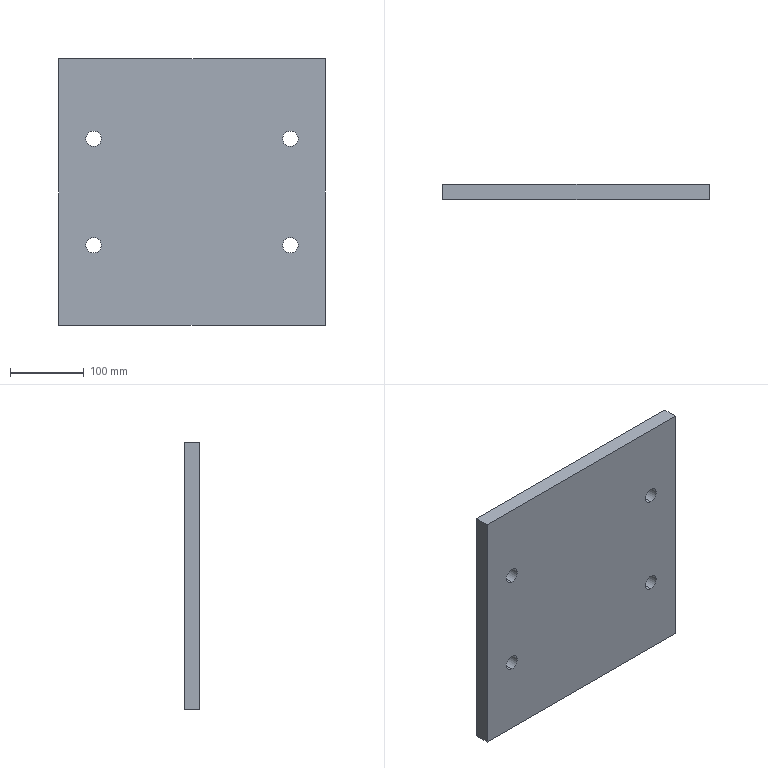Part | SolidWorks | features Extrusion 1, HoleWzd 1, LPattern 1 | 1 solid | 14 faces | box 360 x 20 x 360 mm | volume 2564291 mm3 | cylinder 8 | plane 6 | commonest cylinder face diameters 21 x8
STEP:
#1=CARTESIAN_POINT('',(133.,-10.,61.5));
#2=VERTEX_POINT('',#1);
#3=CARTESIAN_POINT('',(133.,-10.,82.5));
#4=VERTEX_POINT('',#3);
#5=CARTESIAN_POINT('',(133.,-10.,72.));
#6=DIRECTION('',(0.,1.,0.));
#7=DIRECTION('',(0.,0.,1.));
#8=AXIS2_PLACEMENT_3D('',#5,#6,#7);
#9=CIRCLE('',#8,10.5);
#10=EDGE_CURVE('',#2,#4,#9,.T.);
#11=ORIENTED_EDGE('',*,*,#10,.F.);
#12=CARTESIAN_POINT('',(133.,10.,61.5));
#13=VERTEX_POINT('',#12);
#14=CARTESIAN_POINT('',(133.,10.,61.5));
#15=DIRECTION('',(0.,1.,0.));
#16=VECTOR('',#15,1000.);
#17=LINE('',#14,#16);
#18=EDGE_CURVE('',#2,#13,#17,.T.);
#19=ORIENTED_EDGE('',*,*,#18,.T.);
#20=CARTESIAN_POINT('',(133.,10.,82.5));
#21=VERTEX_POINT('',#20);
#22=CARTESIAN_POINT('',(133.,10.,72.));
#23=DIRECTION('',(0.,1.,0.));
#24=DIRECTION('',(0.,0.,1.));
#25=AXIS2_PLACEMENT_3D('',#22,#23,#24);
#26=CIRCLE('',#25,10.5);
#27=EDGE_CURVE('',#13,#21,#26,.T.);
#28=ORIENTED_EDGE('',*,*,#27,.T.);
#29=CARTESIAN_POINT('',(133.,10.,82.5));
#30=DIRECTION('',(0.,1.,0.));
#31=VECTOR('',#30,1000.);
#32=LINE('',#29,#31);
#33=EDGE_CURVE('',#4,#21,#32,.T.);
#34=ORIENTED_EDGE('',*,*,#33,.F.);
#35=EDGE_LOOP('',(#11,#19,#28,#34));
#36=FACE_OUTER_BOUND('',#35,.T.);
#37=CARTESIAN_POINT('',(133.,10.,72.));
#38=DIRECTION('',(0.,1.,0.));
#39=DIRECTION('',(0.,0.,1.));
#40=AXIS2_PLACEMENT_3D('',#37,#38,#39);
#41=CYLINDRICAL_SURFACE('',#40,10.5);
#42=ADVANCED_FACE('',(#36),#41,.F.);
#43=CARTESIAN_POINT('',(133.,-10.,-82.5));
#44=VERTEX_POINT('',#43);
#45=CARTESIAN_POINT('',(133.,-10.,-61.5));
#46=VERTEX_POINT('',#45);
#47=CARTESIAN_POINT('',(133.,-10.,-72.));
#48=DIRECTION('',(0.,1.,0.));
#49=DIRECTION('',(0.,0.,1.));
#50=AXIS2_PLACEMENT_3D('',#47,#48,#49);
#51=CIRCLE('',#50,10.5);
#52=EDGE_CURVE('',#44,#46,#51,.T.);
#53=ORIENTED_EDGE('',*,*,#52,.F.);
#54=CARTESIAN_POINT('',(133.,10.,-82.5));
#55=VERTEX_POINT('',#54);
#56=CARTESIAN_POINT('',(133.,10.,-82.5));
#57=DIRECTION('',(0.,1.,0.));
#58=VECTOR('',#57,1000.);
#59=LINE('',#56,#58);
#60=EDGE_CURVE('',#44,#55,#59,.T.);
#61=ORIENTED_EDGE('',*,*,#60,.T.);
#62=CARTESIAN_POINT('',(133.,10.,-61.5));
#63=VERTEX_POINT('',#62);
#64=CARTESIAN_POINT('',(133.,10.,-72.));
#65=DIRECTION('',(0.,1.,0.));
#66=DIRECTION('',(0.,0.,1.));
#67=AXIS2_PLACEMENT_3D('',#64,#65,#66);
#68=CIRCLE('',#67,10.5);
#69=EDGE_CURVE('',#55,#63,#68,.T.);
#70=ORIENTED_EDGE('',*,*,#69,.T.);
#71=CARTESIAN_POINT('',(133.,10.,-61.5));
#72=DIRECTION('',(0.,1.,0.));
#73=VECTOR('',#72,1000.);
#74=LINE('',#71,#73);
#75=EDGE_CURVE('',#46,#63,#74,.T.);
#76=ORIENTED_EDGE('',*,*,#75,.F.);
#77=EDGE_LOOP('',(#53,#61,#70,#76));
#78=FACE_OUTER_BOUND('',#77,.T.);
#79=CARTESIAN_POINT('',(133.,10.,-72.));
#80=DIRECTION('',(0.,1.,0.));
#81=DIRECTION('',(0.,0.,1.));
#82=AXIS2_PLACEMENT_3D('',#79,#80,#81);
#83=CYLINDRICAL_SURFACE('',#82,10.5);
#84=ADVANCED_FACE('',(#78),#83,.F.);
#85=CARTESIAN_POINT('',(-133.,-10.,61.5));
#86=VERTEX_POINT('',#85);
#87=CARTESIAN_POINT('',(-133.,-10.,82.5));
#88=VERTEX_POINT('',#87);
#89=CARTESIAN_POINT('',(-133.,-10.,72.));
#90=DIRECTION('',(0.,1.,0.));
#91=DIRECTION('',(0.,0.,1.));
#92=AXIS2_PLACEMENT_3D('',#89,#90,#91);
#93=CIRCLE('',#92,10.5);
#94=EDGE_CURVE('',#86,#88,#93,.T.);
#95=ORIENTED_EDGE('',*,*,#94,.F.);
#96=CARTESIAN_POINT('',(-133.,10.,61.5));
#97=VERTEX_POINT('',#96);
#98=CARTESIAN_POINT('',(-133.,10.,61.5));
#99=DIRECTION('',(0.,1.,0.));
#100=VECTOR('',#99,1000.);
#101=LINE('',#98,#100);
#102=EDGE_CURVE('',#86,#97,#101,.T.);
#103=ORIENTED_EDGE('',*,*,#102,.T.);
#104=CARTESIAN_POINT('',(-133.,10.,82.5));
#105=VERTEX_POINT('',#104);
#106=CARTESIAN_POINT('',(-133.,10.,72.));
#107=DIRECTION('',(0.,1.,0.));
#108=DIRECTION('',(0.,0.,1.));
#109=AXIS2_PLACEMENT_3D('',#106,#107,#108);
#110=CIRCLE('',#109,10.5);
#111=EDGE_CURVE('',#97,#105,#110,.T.);
#112=ORIENTED_EDGE('',*,*,#111,.T.);
#113=CARTESIAN_POINT('',(-133.,10.,82.5));
#114=DIRECTION('',(0.,1.,0.));
#115=VECTOR('',#114,1000.);
#116=LINE('',#113,#115);
#117=EDGE_CURVE('',#88,#105,#116,.T.);
#118=ORIENTED_EDGE('',*,*,#117,.F.);
#119=EDGE_LOOP('',(#95,#103,#112,#118));
#120=FACE_OUTER_BOUND('',#119,.T.);
#121=CARTESIAN_POINT('',(-133.,10.,72.));
#122=DIRECTION('',(0.,1.,0.));
#123=DIRECTION('',(0.,0.,1.));
#124=AXIS2_PLACEMENT_3D('',#121,#122,#123);
#125=CYLINDRICAL_SURFACE('',#124,10.5);
#126=ADVANCED_FACE('',(#120),#125,.F.);
#127=CARTESIAN_POINT('',(-133.,-10.,-82.5));
#128=VERTEX_POINT('',#127);
#129=CARTESIAN_POINT('',(-133.,-10.,-61.5));
#130=VERTEX_POINT('',#129);
#131=CARTESIAN_POINT('',(-133.,-10.,-72.));
#132=DIRECTION('',(0.,1.,0.));
#133=DIRECTION('',(0.,0.,1.));
#134=AXIS2_PLACEMENT_3D('',#131,#132,#133);
#135=CIRCLE('',#134,10.5);
#136=EDGE_CURVE('',#128,#130,#135,.T.);
#137=ORIENTED_EDGE('',*,*,#136,.F.);
#138=CARTESIAN_POINT('',(-133.,10.,-82.5));
#139=VERTEX_POINT('',#138);
#140=CARTESIAN_POINT('',(-133.,10.,-82.5));
#141=DIRECTION('',(0.,1.,0.));
#142=VECTOR('',#141,1000.);
#143=LINE('',#140,#142);
#144=EDGE_CURVE('',#128,#139,#143,.T.);
#145=ORIENTED_EDGE('',*,*,#144,.T.);
#146=CARTESIAN_POINT('',(-133.,10.,-61.5));
#147=VERTEX_POINT('',#146);
#148=CARTESIAN_POINT('',(-133.,10.,-72.));
#149=DIRECTION('',(0.,1.,0.));
#150=DIRECTION('',(0.,0.,1.));
#151=AXIS2_PLACEMENT_3D('',#148,#149,#150);
#152=CIRCLE('',#151,10.5);
#153=EDGE_CURVE('',#139,#147,#152,.T.);
#154=ORIENTED_EDGE('',*,*,#153,.T.);
#155=CARTESIAN_POINT('',(-133.,10.,-61.5));
#156=DIRECTION('',(0.,1.,0.));
#157=VECTOR('',#156,1000.);
#158=LINE('',#155,#157);
#159=EDGE_CURVE('',#130,#147,#158,.T.);
#160=ORIENTED_EDGE('',*,*,#159,.F.);
#161=EDGE_LOOP('',(#137,#145,#154,#160));
#162=FACE_OUTER_BOUND('',#161,.T.);
#163=CARTESIAN_POINT('',(-133.,10.,-72.));
#164=DIRECTION('',(0.,1.,0.));
#165=DIRECTION('',(0.,0.,1.));
#166=AXIS2_PLACEMENT_3D('',#163,#164,#165);
#167=CYLINDRICAL_SURFACE('',#166,10.5);
#168=ADVANCED_FACE('',(#162),#167,.F.);
#169=CARTESIAN_POINT('',(180.,-10.,-180.));
#170=VERTEX_POINT('',#169);
#171=CARTESIAN_POINT('',(-180.,-10.,-180.));
#172=VERTEX_POINT('',#171);
#173=CARTESIAN_POINT('',(180.,-10.,-180.));
#174=DIRECTION('',(-1.,0.,0.));
#175=VECTOR('',#174,1000.);
#176=LINE('',#173,#175);
#177=EDGE_CURVE('',#170,#172,#176,.T.);
#178=ORIENTED_EDGE('',*,*,#177,.T.);
#179=CARTESIAN_POINT('',(-180.,10.,-180.));
#180=VERTEX_POINT('',#179);
#181=CARTESIAN_POINT('',(-180.,10.,-180.));
#182=DIRECTION('',(0.,-1.,0.));
#183=VECTOR('',#182,1000.);
#184=LINE('',#181,#183);
#185=EDGE_CURVE('',#180,#172,#184,.T.);
#186=ORIENTED_EDGE('',*,*,#185,.F.);
#187=CARTESIAN_POINT('',(180.,10.,-180.));
#188=VERTEX_POINT('',#187);
#189=CARTESIAN_POINT('',(180.,10.,-180.));
#190=DIRECTION('',(-1.,0.,0.));
#191=VECTOR('',#190,1000.);
#192=LINE('',#189,#191);
#193=EDGE_CURVE('',#188,#180,#192,.T.);
#194=ORIENTED_EDGE('',*,*,#193,.F.);
#195=CARTESIAN_POINT('',(180.,10.,-180.));
#196=DIRECTION('',(0.,-1.,0.));
#197=VECTOR('',#196,1000.);
#198=LINE('',#195,#197);
#199=EDGE_CURVE('',#188,#170,#198,.T.);
#200=ORIENTED_EDGE('',*,*,#199,.T.);
#201=EDGE_LOOP('',(#178,#186,#194,#200));
#202=FACE_OUTER_BOUND('',#201,.T.);
#203=CARTESIAN_POINT('',(180.,10.,-180.));
#204=DIRECTION('',(0.,0.,1.));
#205=DIRECTION('',(1.,0.,0.));
#206=AXIS2_PLACEMENT_3D('',#203,#204,#205);
#207=PLANE('',#206);
#208=ADVANCED_FACE('',(#202),#207,.F.);
#209=CARTESIAN_POINT('',(-180.,-10.,180.));
#210=VERTEX_POINT('',#209);
#211=CARTESIAN_POINT('',(-180.,-10.,-180.));
#212=DIRECTION('',(0.,0.,1.));
#213=VECTOR('',#212,1000.);
#214=LINE('',#211,#213);
#215=EDGE_CURVE('',#172,#210,#214,.T.);
#216=ORIENTED_EDGE('',*,*,#215,.T.);
#217=CARTESIAN_POINT('',(-180.,10.,180.));
#218=VERTEX_POINT('',#217);
#219=CARTESIAN_POINT('',(-180.,10.,180.));
#220=DIRECTION('',(0.,-1.,0.));
#221=VECTOR('',#220,1000.);
#222=LINE('',#219,#221);
#223=EDGE_CURVE('',#218,#210,#222,.T.);
#224=ORIENTED_EDGE('',*,*,#223,.F.);
#225=CARTESIAN_POINT('',(-180.,10.,-180.));
#226=DIRECTION('',(0.,0.,1.));
#227=VECTOR('',#226,1000.);
#228=LINE('',#225,#227);
#229=EDGE_CURVE('',#180,#218,#228,.T.);
#230=ORIENTED_EDGE('',*,*,#229,.F.);
#231=ORIENTED_EDGE('',*,*,#185,.T.);
#232=EDGE_LOOP('',(#216,#224,#230,#231));
#233=FACE_OUTER_BOUND('',#232,.T.);
#234=CARTESIAN_POINT('',(-180.,10.,-180.));
#235=DIRECTION('',(1.,0.,0.));
#236=DIRECTION('',(0.,0.,-1.));
#237=AXIS2_PLACEMENT_3D('',#234,#235,#236);
#238=PLANE('',#237);
#239=ADVANCED_FACE('',(#233),#238,.F.);
#240=CARTESIAN_POINT('',(180.,-10.,180.));
#241=VERTEX_POINT('',#240);
#242=CARTESIAN_POINT('',(-180.,-10.,180.));
#243=DIRECTION('',(1.,0.,0.));
#244=VECTOR('',#243,1000.);
#245=LINE('',#242,#244);
#246=EDGE_CURVE('',#210,#241,#245,.T.);
#247=ORIENTED_EDGE('',*,*,#246,.T.);
#248=CARTESIAN_POINT('',(180.,10.,180.));
#249=VERTEX_POINT('',#248);
#250=CARTESIAN_POINT('',(180.,10.,180.));
#251=DIRECTION('',(0.,-1.,0.));
#252=VECTOR('',#251,1000.);
#253=LINE('',#250,#252);
#254=EDGE_CURVE('',#249,#241,#253,.T.);
#255=ORIENTED_EDGE('',*,*,#254,.F.);
#256=CARTESIAN_POINT('',(-180.,10.,180.));
#257=DIRECTION('',(1.,0.,0.));
#258=VECTOR('',#257,1000.);
#259=LINE('',#256,#258);
#260=EDGE_CURVE('',#218,#249,#259,.T.);
#261=ORIENTED_EDGE('',*,*,#260,.F.);
#262=ORIENTED_EDGE('',*,*,#223,.T.);
#263=EDGE_LOOP('',(#247,#255,#261,#262));
#264=FACE_OUTER_BOUND('',#263,.T.);
#265=CARTESIAN_POINT('',(-180.,10.,180.));
#266=DIRECTION('',(0.,0.,-1.));
#267=DIRECTION('',(-1.,0.,0.));
#268=AXIS2_PLACEMENT_3D('',#265,#266,#267);
#269=PLANE('',#268);
#270=ADVANCED_FACE('',(#264),#269,.F.);
#271=CARTESIAN_POINT('',(180.,-10.,180.));
#272=DIRECTION('',(0.,0.,-1.));
#273=VECTOR('',#272,1000.);
#274=LINE('',#271,#273);
#275=EDGE_CURVE('',#241,#170,#274,.T.);
#276=ORIENTED_EDGE('',*,*,#275,.T.);
#277=ORIENTED_EDGE('',*,*,#199,.F.);
#278=CARTESIAN_POINT('',(180.,10.,180.));
#279=DIRECTION('',(0.,0.,-1.));
#280=VECTOR('',#279,1000.);
#281=LINE('',#278,#280);
#282=EDGE_CURVE('',#249,#188,#281,.T.);
#283=ORIENTED_EDGE('',*,*,#282,.F.);
#284=ORIENTED_EDGE('',*,*,#254,.T.);
#285=EDGE_LOOP('',(#276,#277,#283,#284));
#286=FACE_OUTER_BOUND('',#285,.T.);
#287=CARTESIAN_POINT('',(180.,10.,180.));
#288=DIRECTION('',(-1.,0.,0.));
#289=DIRECTION('',(0.,0.,1.));
#290=AXIS2_PLACEMENT_3D('',#287,#288,#289);
#291=PLANE('',#290);
#292=ADVANCED_FACE('',(#286),#291,.F.);
#293=CARTESIAN_POINT('',(-133.,10.,72.));
#294=DIRECTION('',(0.,1.,0.));
#295=DIRECTION('',(0.,0.,1.));
#296=AXIS2_PLACEMENT_3D('',#293,#294,#295);
#297=CIRCLE('',#296,10.5);
#298=EDGE_CURVE('',#105,#97,#297,.T.);
#299=ORIENTED_EDGE('',*,*,#298,.F.);
#300=ORIENTED_EDGE('',*,*,#111,.F.);
#301=EDGE_LOOP('',(#299,#300));
#302=FACE_BOUND('',#301,.T.);
#303=CARTESIAN_POINT('',(-133.,10.,-72.));
#304=DIRECTION('',(0.,1.,0.));
#305=DIRECTION('',(0.,0.,1.));
#306=AXIS2_PLACEMENT_3D('',#303,#304,#305);
#307=CIRCLE('',#306,10.5);
#308=EDGE_CURVE('',#147,#139,#307,.T.);
#309=ORIENTED_EDGE('',*,*,#308,.F.);
#310=ORIENTED_EDGE('',*,*,#153,.F.);
#311=EDGE_LOOP('',(#309,#310));
#312=FACE_BOUND('',#311,.T.);
#313=ORIENTED_EDGE('',*,*,#193,.T.);
#314=ORIENTED_EDGE('',*,*,#229,.T.);
#315=ORIENTED_EDGE('',*,*,#260,.T.);
#316=ORIENTED_EDGE('',*,*,#282,.T.);
#317=EDGE_LOOP('',(#313,#314,#315,#316));
#318=FACE_OUTER_BOUND('',#317,.T.);
#319=CARTESIAN_POINT('',(133.,10.,-72.));
#320=DIRECTION('',(0.,1.,0.));
#321=DIRECTION('',(0.,0.,1.));
#322=AXIS2_PLACEMENT_3D('',#319,#320,#321);
#323=CIRCLE('',#322,10.5);
#324=EDGE_CURVE('',#63,#55,#323,.T.);
#325=ORIENTED_EDGE('',*,*,#324,.F.);
#326=ORIENTED_EDGE('',*,*,#69,.F.);
#327=EDGE_LOOP('',(#325,#326));
#328=FACE_BOUND('',#327,.T.);
#329=CARTESIAN_POINT('',(133.,10.,72.));
#330=DIRECTION('',(0.,1.,0.));
#331=DIRECTION('',(0.,0.,1.));
#332=AXIS2_PLACEMENT_3D('',#329,#330,#331);
#333=CIRCLE('',#332,10.5);
#334=EDGE_CURVE('',#21,#13,#333,.T.);
#335=ORIENTED_EDGE('',*,*,#334,.F.);
#336=ORIENTED_EDGE('',*,*,#27,.F.);
#337=EDGE_LOOP('',(#335,#336));
#338=FACE_BOUND('',#337,.T.);
#339=CARTESIAN_POINT('',(-180.,10.,-180.));
#340=DIRECTION('',(0.,1.,0.));
#341=DIRECTION('',(0.,0.,1.));
#342=AXIS2_PLACEMENT_3D('',#339,#340,#341);
#343=PLANE('',#342);
#344=ADVANCED_FACE('',(#302,#312,#318,#328,#338),#343,.T.);
#345=CARTESIAN_POINT('',(-133.,-10.,72.));
#346=DIRECTION('',(0.,1.,0.));
#347=DIRECTION('',(0.,0.,1.));
#348=AXIS2_PLACEMENT_3D('',#345,#346,#347);
#349=CIRCLE('',#348,10.5);
#350=EDGE_CURVE('',#88,#86,#349,.T.);
#351=ORIENTED_EDGE('',*,*,#350,.T.);
#352=ORIENTED_EDGE('',*,*,#94,.T.);
#353=EDGE_LOOP('',(#351,#352));
#354=FACE_BOUND('',#353,.T.);
#355=CARTESIAN_POINT('',(-133.,-10.,-72.));
#356=DIRECTION('',(0.,1.,0.));
#357=DIRECTION('',(0.,0.,1.));
#358=AXIS2_PLACEMENT_3D('',#355,#356,#357);
#359=CIRCLE('',#358,10.5);
#360=EDGE_CURVE('',#130,#128,#359,.T.);
#361=ORIENTED_EDGE('',*,*,#360,.T.);
#362=ORIENTED_EDGE('',*,*,#136,.T.);
#363=EDGE_LOOP('',(#361,#362));
#364=FACE_BOUND('',#363,.T.);
#365=ORIENTED_EDGE('',*,*,#177,.F.);
#366=ORIENTED_EDGE('',*,*,#275,.F.);
#367=ORIENTED_EDGE('',*,*,#246,.F.);
#368=ORIENTED_EDGE('',*,*,#215,.F.);
#369=EDGE_LOOP('',(#365,#366,#367,#368));
#370=FACE_OUTER_BOUND('',#369,.T.);
#371=CARTESIAN_POINT('',(133.,-10.,-72.));
#372=DIRECTION('',(0.,1.,0.));
#373=DIRECTION('',(0.,0.,1.));
#374=AXIS2_PLACEMENT_3D('',#371,#372,#373);
#375=CIRCLE('',#374,10.5);
#376=EDGE_CURVE('',#46,#44,#375,.T.);
#377=ORIENTED_EDGE('',*,*,#376,.T.);
#378=ORIENTED_EDGE('',*,*,#52,.T.);
#379=EDGE_LOOP('',(#377,#378));
#380=FACE_BOUND('',#379,.T.);
#381=CARTESIAN_POINT('',(133.,-10.,72.));
#382=DIRECTION('',(0.,1.,0.));
#383=DIRECTION('',(0.,0.,1.));
#384=AXIS2_PLACEMENT_3D('',#381,#382,#383);
#385=CIRCLE('',#384,10.5);
#386=EDGE_CURVE('',#4,#2,#385,.T.);
#387=ORIENTED_EDGE('',*,*,#386,.T.);
#388=ORIENTED_EDGE('',*,*,#10,.T.);
#389=EDGE_LOOP('',(#387,#388));
#390=FACE_BOUND('',#389,.T.);
#391=CARTESIAN_POINT('',(-180.,-10.,-180.));
#392=DIRECTION('',(0.,1.,0.));
#393=DIRECTION('',(0.,0.,1.));
#394=AXIS2_PLACEMENT_3D('',#391,#392,#393);
#395=PLANE('',#394);
#396=ADVANCED_FACE('',(#354,#364,#370,#380,#390),#395,.F.);
#397=ORIENTED_EDGE('',*,*,#144,.F.);
#398=ORIENTED_EDGE('',*,*,#360,.F.);
#399=ORIENTED_EDGE('',*,*,#159,.T.);
#400=ORIENTED_EDGE('',*,*,#308,.T.);
#401=EDGE_LOOP('',(#397,#398,#399,#400));
#402=FACE_OUTER_BOUND('',#401,.T.);
#403=CARTESIAN_POINT('',(-133.,10.,-72.));
#404=DIRECTION('',(0.,1.,0.));
#405=DIRECTION('',(0.,0.,1.));
#406=AXIS2_PLACEMENT_3D('',#403,#404,#405);
#407=CYLINDRICAL_SURFACE('',#406,10.5);
#408=ADVANCED_FACE('',(#402),#407,.F.);
#409=ORIENTED_EDGE('',*,*,#102,.F.);
#410=ORIENTED_EDGE('',*,*,#350,.F.);
#411=ORIENTED_EDGE('',*,*,#117,.T.);
#412=ORIENTED_EDGE('',*,*,#298,.T.);
#413=EDGE_LOOP('',(#409,#410,#411,#412));
#414=FACE_OUTER_BOUND('',#413,.T.);
#415=CARTESIAN_POINT('',(-133.,10.,72.));
#416=DIRECTION('',(0.,1.,0.));
#417=DIRECTION('',(0.,0.,1.));
#418=AXIS2_PLACEMENT_3D('',#415,#416,#417);
#419=CYLINDRICAL_SURFACE('',#418,10.5);
#420=ADVANCED_FACE('',(#414),#419,.F.);
#421=ORIENTED_EDGE('',*,*,#60,.F.);
#422=ORIENTED_EDGE('',*,*,#376,.F.);
#423=ORIENTED_EDGE('',*,*,#75,.T.);
#424=ORIENTED_EDGE('',*,*,#324,.T.);
#425=EDGE_LOOP('',(#421,#422,#423,#424));
#426=FACE_OUTER_BOUND('',#425,.T.);
#427=CARTESIAN_POINT('',(133.,10.,-72.));
#428=DIRECTION('',(0.,1.,0.));
#429=DIRECTION('',(0.,0.,1.));
#430=AXIS2_PLACEMENT_3D('',#427,#428,#429);
#431=CYLINDRICAL_SURFACE('',#430,10.5);
#432=ADVANCED_FACE('',(#426),#431,.F.);
#433=ORIENTED_EDGE('',*,*,#18,.F.);
#434=ORIENTED_EDGE('',*,*,#386,.F.);
#435=ORIENTED_EDGE('',*,*,#33,.T.);
#436=ORIENTED_EDGE('',*,*,#334,.T.);
#437=EDGE_LOOP('',(#433,#434,#435,#436));
#438=FACE_OUTER_BOUND('',#437,.T.);
#439=CARTESIAN_POINT('',(133.,10.,72.));
#440=DIRECTION('',(0.,1.,0.));
#441=DIRECTION('',(0.,0.,1.));
#442=AXIS2_PLACEMENT_3D('',#439,#440,#441);
#443=CYLINDRICAL_SURFACE('',#442,10.5);
#444=ADVANCED_FACE('',(#438),#443,.F.);
#445=CLOSED_SHELL('',(#42,#84,#126,#168,#208,#239,#270,#292,#344,#396,#408,#420,#432,#444));
#446=MANIFOLD_SOLID_BREP('',#445);
#447=CARTESIAN_POINT('',(0.,0.,0.));
#448=DIRECTION('',(0.,0.,1.));
#449=DIRECTION('',(1.,0.,0.));
#450=AXIS2_PLACEMENT_3D('',#447,#448,#449);
#451=(LENGTH_UNIT()NAMED_UNIT(*)SI_UNIT(.MILLI.,.METRE.));
#452=UNCERTAINTY_MEASURE_WITH_UNIT(LENGTH_MEASURE(0.00001),#451,'','');
#453=(NAMED_UNIT(*)PLANE_ANGLE_UNIT()SI_UNIT($,.RADIAN.));
#454=(NAMED_UNIT(*)SI_UNIT($,.STERADIAN.)SOLID_ANGLE_UNIT());
#455=(GEOMETRIC_REPRESENTATION_CONTEXT(3)GLOBAL_UNCERTAINTY_ASSIGNED_CONTEXT((#452))GLOBAL_UNIT_ASSIGNED_CONTEXT((#451,#453,#454))REPRESENTATION_CONTEXT('',''));
#456=ADVANCED_BREP_SHAPE_REPRESENTATION('',(#446,#450),#455);